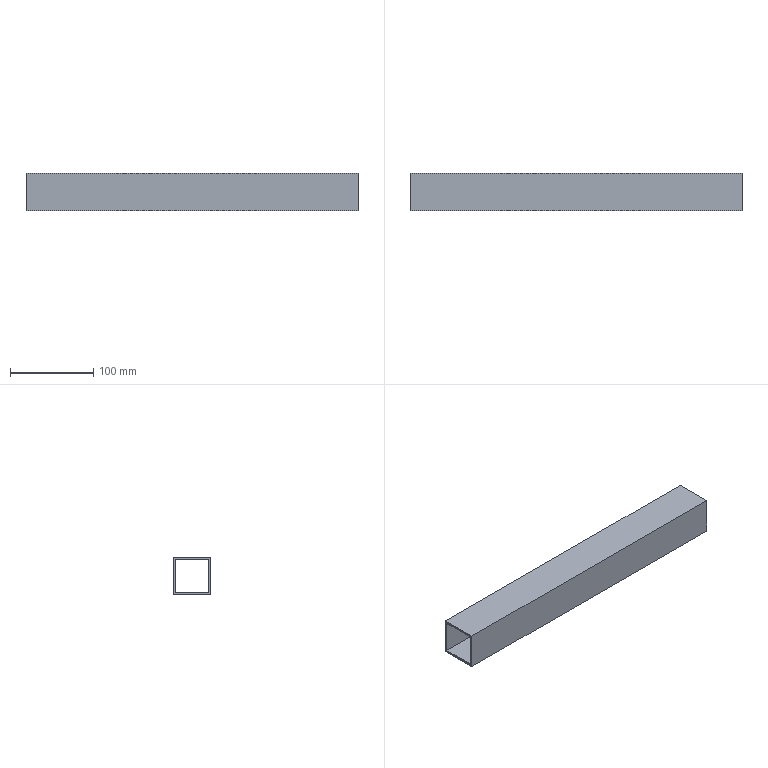Part | STEP file | MB-360X400 | 1 solid | 10 faces | box 400 x 45 x 45 mm | volume 170000 mm3 | plane 10
STEP:
#1=CARTESIAN_POINT('',(0.,42.5,2.5));
#2=VERTEX_POINT('',#1);
#3=CARTESIAN_POINT('',(0.,2.5,2.5));
#4=VERTEX_POINT('',#3);
#5=CARTESIAN_POINT('',(0.,2.5,2.5));
#6=DIRECTION('',(0.,-1.,0.));
#7=VECTOR('',#6,1000.);
#8=LINE('',#5,#7);
#9=EDGE_CURVE('',#2,#4,#8,.T.);
#10=ORIENTED_EDGE('',*,*,#9,.F.);
#11=CARTESIAN_POINT('',(0.,42.5,42.5));
#12=VERTEX_POINT('',#11);
#13=CARTESIAN_POINT('',(0.,42.5,2.5));
#14=DIRECTION('',(0.,0.,-1.));
#15=VECTOR('',#14,1000.);
#16=LINE('',#13,#15);
#17=EDGE_CURVE('',#12,#2,#16,.T.);
#18=ORIENTED_EDGE('',*,*,#17,.F.);
#19=CARTESIAN_POINT('',(0.,2.5,42.5));
#20=VERTEX_POINT('',#19);
#21=CARTESIAN_POINT('',(0.,42.5,42.5));
#22=DIRECTION('',(0.,1.,0.));
#23=VECTOR('',#22,1000.);
#24=LINE('',#21,#23);
#25=EDGE_CURVE('',#20,#12,#24,.T.);
#26=ORIENTED_EDGE('',*,*,#25,.F.);
#27=CARTESIAN_POINT('',(0.,2.5,42.5));
#28=DIRECTION('',(0.,0.,1.));
#29=VECTOR('',#28,1000.);
#30=LINE('',#27,#29);
#31=EDGE_CURVE('',#4,#20,#30,.T.);
#32=ORIENTED_EDGE('',*,*,#31,.F.);
#33=EDGE_LOOP('',(#10,#18,#26,#32));
#34=FACE_BOUND('',#33,.T.);
#35=CARTESIAN_POINT('',(0.,0.,45.));
#36=VERTEX_POINT('',#35);
#37=CARTESIAN_POINT('',(0.,0.,0.));
#38=VERTEX_POINT('',#37);
#39=CARTESIAN_POINT('',(0.,0.,45.));
#40=DIRECTION('',(0.,0.,-1.));
#41=VECTOR('',#40,1000.);
#42=LINE('',#39,#41);
#43=EDGE_CURVE('',#36,#38,#42,.T.);
#44=ORIENTED_EDGE('',*,*,#43,.F.);
#45=CARTESIAN_POINT('',(0.,45.,45.));
#46=VERTEX_POINT('',#45);
#47=CARTESIAN_POINT('',(0.,45.,45.));
#48=DIRECTION('',(0.,-1.,0.));
#49=VECTOR('',#48,1000.);
#50=LINE('',#47,#49);
#51=EDGE_CURVE('',#46,#36,#50,.T.);
#52=ORIENTED_EDGE('',*,*,#51,.F.);
#53=CARTESIAN_POINT('',(0.,45.,0.));
#54=VERTEX_POINT('',#53);
#55=CARTESIAN_POINT('',(0.,45.,0.));
#56=DIRECTION('',(0.,0.,1.));
#57=VECTOR('',#56,1000.);
#58=LINE('',#55,#57);
#59=EDGE_CURVE('',#54,#46,#58,.T.);
#60=ORIENTED_EDGE('',*,*,#59,.F.);
#61=CARTESIAN_POINT('',(0.,0.,0.));
#62=DIRECTION('',(0.,1.,0.));
#63=VECTOR('',#62,1000.);
#64=LINE('',#61,#63);
#65=EDGE_CURVE('',#38,#54,#64,.T.);
#66=ORIENTED_EDGE('',*,*,#65,.F.);
#67=EDGE_LOOP('',(#44,#52,#60,#66));
#68=FACE_OUTER_BOUND('',#67,.T.);
#69=CARTESIAN_POINT('',(0.,22.5,22.5));
#70=DIRECTION('',(1.,0.,0.));
#71=DIRECTION('',(0.,1.,0.));
#72=AXIS2_PLACEMENT_3D('',#69,#70,#71);
#73=PLANE('',#72);
#74=ADVANCED_FACE('',(#34,#68),#73,.F.);
#75=CARTESIAN_POINT('',(400.,42.5,2.5));
#76=VERTEX_POINT('',#75);
#77=CARTESIAN_POINT('',(400.,2.5,2.5));
#78=VERTEX_POINT('',#77);
#79=CARTESIAN_POINT('',(400.,2.5,2.5));
#80=DIRECTION('',(0.,-1.,0.));
#81=VECTOR('',#80,1000.);
#82=LINE('',#79,#81);
#83=EDGE_CURVE('',#76,#78,#82,.T.);
#84=ORIENTED_EDGE('',*,*,#83,.T.);
#85=CARTESIAN_POINT('',(400.,2.5,42.5));
#86=VERTEX_POINT('',#85);
#87=CARTESIAN_POINT('',(400.,2.5,42.5));
#88=DIRECTION('',(0.,0.,1.));
#89=VECTOR('',#88,1000.);
#90=LINE('',#87,#89);
#91=EDGE_CURVE('',#78,#86,#90,.T.);
#92=ORIENTED_EDGE('',*,*,#91,.T.);
#93=CARTESIAN_POINT('',(400.,42.5,42.5));
#94=VERTEX_POINT('',#93);
#95=CARTESIAN_POINT('',(400.,42.5,42.5));
#96=DIRECTION('',(0.,1.,0.));
#97=VECTOR('',#96,1000.);
#98=LINE('',#95,#97);
#99=EDGE_CURVE('',#86,#94,#98,.T.);
#100=ORIENTED_EDGE('',*,*,#99,.T.);
#101=CARTESIAN_POINT('',(400.,42.5,2.5));
#102=DIRECTION('',(0.,0.,-1.));
#103=VECTOR('',#102,1000.);
#104=LINE('',#101,#103);
#105=EDGE_CURVE('',#94,#76,#104,.T.);
#106=ORIENTED_EDGE('',*,*,#105,.T.);
#107=EDGE_LOOP('',(#84,#92,#100,#106));
#108=FACE_BOUND('',#107,.T.);
#109=CARTESIAN_POINT('',(400.,0.,45.));
#110=VERTEX_POINT('',#109);
#111=CARTESIAN_POINT('',(400.,0.,0.));
#112=VERTEX_POINT('',#111);
#113=CARTESIAN_POINT('',(400.,0.,45.));
#114=DIRECTION('',(0.,0.,-1.));
#115=VECTOR('',#114,1000.);
#116=LINE('',#113,#115);
#117=EDGE_CURVE('',#110,#112,#116,.T.);
#118=ORIENTED_EDGE('',*,*,#117,.T.);
#119=CARTESIAN_POINT('',(400.,45.,0.));
#120=VERTEX_POINT('',#119);
#121=CARTESIAN_POINT('',(400.,0.,0.));
#122=DIRECTION('',(0.,1.,0.));
#123=VECTOR('',#122,1000.);
#124=LINE('',#121,#123);
#125=EDGE_CURVE('',#112,#120,#124,.T.);
#126=ORIENTED_EDGE('',*,*,#125,.T.);
#127=CARTESIAN_POINT('',(400.,45.,45.));
#128=VERTEX_POINT('',#127);
#129=CARTESIAN_POINT('',(400.,45.,0.));
#130=DIRECTION('',(0.,0.,1.));
#131=VECTOR('',#130,1000.);
#132=LINE('',#129,#131);
#133=EDGE_CURVE('',#120,#128,#132,.T.);
#134=ORIENTED_EDGE('',*,*,#133,.T.);
#135=CARTESIAN_POINT('',(400.,45.,45.));
#136=DIRECTION('',(0.,-1.,0.));
#137=VECTOR('',#136,1000.);
#138=LINE('',#135,#137);
#139=EDGE_CURVE('',#128,#110,#138,.T.);
#140=ORIENTED_EDGE('',*,*,#139,.T.);
#141=EDGE_LOOP('',(#118,#126,#134,#140));
#142=FACE_OUTER_BOUND('',#141,.T.);
#143=CARTESIAN_POINT('',(400.,22.5,22.5));
#144=DIRECTION('',(1.,0.,0.));
#145=DIRECTION('',(0.,1.,0.));
#146=AXIS2_PLACEMENT_3D('',#143,#144,#145);
#147=PLANE('',#146);
#148=ADVANCED_FACE('',(#108,#142),#147,.T.);
#149=ORIENTED_EDGE('',*,*,#43,.T.);
#150=CARTESIAN_POINT('',(0.,0.,0.));
#151=DIRECTION('',(1.,0.,0.));
#152=VECTOR('',#151,1000.);
#153=LINE('',#150,#152);
#154=EDGE_CURVE('',#38,#112,#153,.T.);
#155=ORIENTED_EDGE('',*,*,#154,.T.);
#156=ORIENTED_EDGE('',*,*,#117,.F.);
#157=CARTESIAN_POINT('',(0.,0.,45.));
#158=DIRECTION('',(1.,0.,0.));
#159=VECTOR('',#158,1000.);
#160=LINE('',#157,#159);
#161=EDGE_CURVE('',#36,#110,#160,.T.);
#162=ORIENTED_EDGE('',*,*,#161,.F.);
#163=EDGE_LOOP('',(#149,#155,#156,#162));
#164=FACE_OUTER_BOUND('',#163,.T.);
#165=CARTESIAN_POINT('',(0.,0.,45.));
#166=DIRECTION('',(0.,-1.,0.));
#167=DIRECTION('',(0.,0.,-1.));
#168=AXIS2_PLACEMENT_3D('',#165,#166,#167);
#169=PLANE('',#168);
#170=ADVANCED_FACE('',(#164),#169,.T.);
#171=ORIENTED_EDGE('',*,*,#65,.T.);
#172=CARTESIAN_POINT('',(0.,45.,0.));
#173=DIRECTION('',(1.,0.,0.));
#174=VECTOR('',#173,1000.);
#175=LINE('',#172,#174);
#176=EDGE_CURVE('',#54,#120,#175,.T.);
#177=ORIENTED_EDGE('',*,*,#176,.T.);
#178=ORIENTED_EDGE('',*,*,#125,.F.);
#179=ORIENTED_EDGE('',*,*,#154,.F.);
#180=EDGE_LOOP('',(#171,#177,#178,#179));
#181=FACE_OUTER_BOUND('',#180,.T.);
#182=CARTESIAN_POINT('',(0.,0.,0.));
#183=DIRECTION('',(0.,0.,-1.));
#184=DIRECTION('',(0.,-1.,0.));
#185=AXIS2_PLACEMENT_3D('',#182,#183,#184);
#186=PLANE('',#185);
#187=ADVANCED_FACE('',(#181),#186,.T.);
#188=ORIENTED_EDGE('',*,*,#59,.T.);
#189=CARTESIAN_POINT('',(0.,45.,45.));
#190=DIRECTION('',(1.,0.,0.));
#191=VECTOR('',#190,1000.);
#192=LINE('',#189,#191);
#193=EDGE_CURVE('',#46,#128,#192,.T.);
#194=ORIENTED_EDGE('',*,*,#193,.T.);
#195=ORIENTED_EDGE('',*,*,#133,.F.);
#196=ORIENTED_EDGE('',*,*,#176,.F.);
#197=EDGE_LOOP('',(#188,#194,#195,#196));
#198=FACE_OUTER_BOUND('',#197,.T.);
#199=CARTESIAN_POINT('',(0.,45.,0.));
#200=DIRECTION('',(0.,1.,0.));
#201=DIRECTION('',(1.,0.,0.));
#202=AXIS2_PLACEMENT_3D('',#199,#200,#201);
#203=PLANE('',#202);
#204=ADVANCED_FACE('',(#198),#203,.T.);
#205=ORIENTED_EDGE('',*,*,#51,.T.);
#206=ORIENTED_EDGE('',*,*,#161,.T.);
#207=ORIENTED_EDGE('',*,*,#139,.F.);
#208=ORIENTED_EDGE('',*,*,#193,.F.);
#209=EDGE_LOOP('',(#205,#206,#207,#208));
#210=FACE_OUTER_BOUND('',#209,.T.);
#211=CARTESIAN_POINT('',(0.,45.,45.));
#212=DIRECTION('',(0.,0.,1.));
#213=DIRECTION('',(1.,0.,0.));
#214=AXIS2_PLACEMENT_3D('',#211,#212,#213);
#215=PLANE('',#214);
#216=ADVANCED_FACE('',(#210),#215,.T.);
#217=ORIENTED_EDGE('',*,*,#9,.T.);
#218=CARTESIAN_POINT('',(0.,2.5,2.5));
#219=DIRECTION('',(1.,0.,0.));
#220=VECTOR('',#219,1000.);
#221=LINE('',#218,#220);
#222=EDGE_CURVE('',#4,#78,#221,.T.);
#223=ORIENTED_EDGE('',*,*,#222,.T.);
#224=ORIENTED_EDGE('',*,*,#83,.F.);
#225=CARTESIAN_POINT('',(0.,42.5,2.5));
#226=DIRECTION('',(1.,0.,0.));
#227=VECTOR('',#226,1000.);
#228=LINE('',#225,#227);
#229=EDGE_CURVE('',#2,#76,#228,.T.);
#230=ORIENTED_EDGE('',*,*,#229,.F.);
#231=EDGE_LOOP('',(#217,#223,#224,#230));
#232=FACE_OUTER_BOUND('',#231,.T.);
#233=CARTESIAN_POINT('',(0.,42.5,2.5));
#234=DIRECTION('',(0.,0.,1.));
#235=DIRECTION('',(1.,0.,0.));
#236=AXIS2_PLACEMENT_3D('',#233,#234,#235);
#237=PLANE('',#236);
#238=ADVANCED_FACE('',(#232),#237,.T.);
#239=ORIENTED_EDGE('',*,*,#31,.T.);
#240=CARTESIAN_POINT('',(0.,2.5,42.5));
#241=DIRECTION('',(1.,0.,0.));
#242=VECTOR('',#241,1000.);
#243=LINE('',#240,#242);
#244=EDGE_CURVE('',#20,#86,#243,.T.);
#245=ORIENTED_EDGE('',*,*,#244,.T.);
#246=ORIENTED_EDGE('',*,*,#91,.F.);
#247=ORIENTED_EDGE('',*,*,#222,.F.);
#248=EDGE_LOOP('',(#239,#245,#246,#247));
#249=FACE_OUTER_BOUND('',#248,.T.);
#250=CARTESIAN_POINT('',(0.,2.5,2.5));
#251=DIRECTION('',(0.,1.,0.));
#252=DIRECTION('',(1.,0.,0.));
#253=AXIS2_PLACEMENT_3D('',#250,#251,#252);
#254=PLANE('',#253);
#255=ADVANCED_FACE('',(#249),#254,.T.);
#256=ORIENTED_EDGE('',*,*,#25,.T.);
#257=CARTESIAN_POINT('',(0.,42.5,42.5));
#258=DIRECTION('',(1.,0.,0.));
#259=VECTOR('',#258,1000.);
#260=LINE('',#257,#259);
#261=EDGE_CURVE('',#12,#94,#260,.T.);
#262=ORIENTED_EDGE('',*,*,#261,.T.);
#263=ORIENTED_EDGE('',*,*,#99,.F.);
#264=ORIENTED_EDGE('',*,*,#244,.F.);
#265=EDGE_LOOP('',(#256,#262,#263,#264));
#266=FACE_OUTER_BOUND('',#265,.T.);
#267=CARTESIAN_POINT('',(0.,2.5,42.5));
#268=DIRECTION('',(0.,0.,-1.));
#269=DIRECTION('',(0.,-1.,0.));
#270=AXIS2_PLACEMENT_3D('',#267,#268,#269);
#271=PLANE('',#270);
#272=ADVANCED_FACE('',(#266),#271,.T.);
#273=ORIENTED_EDGE('',*,*,#17,.T.);
#274=ORIENTED_EDGE('',*,*,#229,.T.);
#275=ORIENTED_EDGE('',*,*,#105,.F.);
#276=ORIENTED_EDGE('',*,*,#261,.F.);
#277=EDGE_LOOP('',(#273,#274,#275,#276));
#278=FACE_OUTER_BOUND('',#277,.T.);
#279=CARTESIAN_POINT('',(0.,42.5,42.5));
#280=DIRECTION('',(0.,-1.,0.));
#281=DIRECTION('',(0.,0.,-1.));
#282=AXIS2_PLACEMENT_3D('',#279,#280,#281);
#283=PLANE('',#282);
#284=ADVANCED_FACE('',(#278),#283,.T.);
#285=CLOSED_SHELL('',(#74,#148,#170,#187,#204,#216,#238,#255,#272,#284));
#286=MANIFOLD_SOLID_BREP('',#285);
#287=CARTESIAN_POINT('',(0.,0.,0.));
#288=DIRECTION('',(0.,0.,1.));
#289=DIRECTION('',(1.,0.,0.));
#290=AXIS2_PLACEMENT_3D('',#287,#288,#289);
#291=(LENGTH_UNIT()NAMED_UNIT(*)SI_UNIT(.MILLI.,.METRE.));
#292=UNCERTAINTY_MEASURE_WITH_UNIT(LENGTH_MEASURE(0.00001),#291,'','');
#293=(NAMED_UNIT(*)PLANE_ANGLE_UNIT()SI_UNIT($,.RADIAN.));
#294=(NAMED_UNIT(*)SI_UNIT($,.STERADIAN.)SOLID_ANGLE_UNIT());
#295=(GEOMETRIC_REPRESENTATION_CONTEXT(3)GLOBAL_UNCERTAINTY_ASSIGNED_CONTEXT((#292))GLOBAL_UNIT_ASSIGNED_CONTEXT((#291,#293,#294))REPRESENTATION_CONTEXT('',''));
#296=ADVANCED_BREP_SHAPE_REPRESENTATION('',(#286,#290),#295);